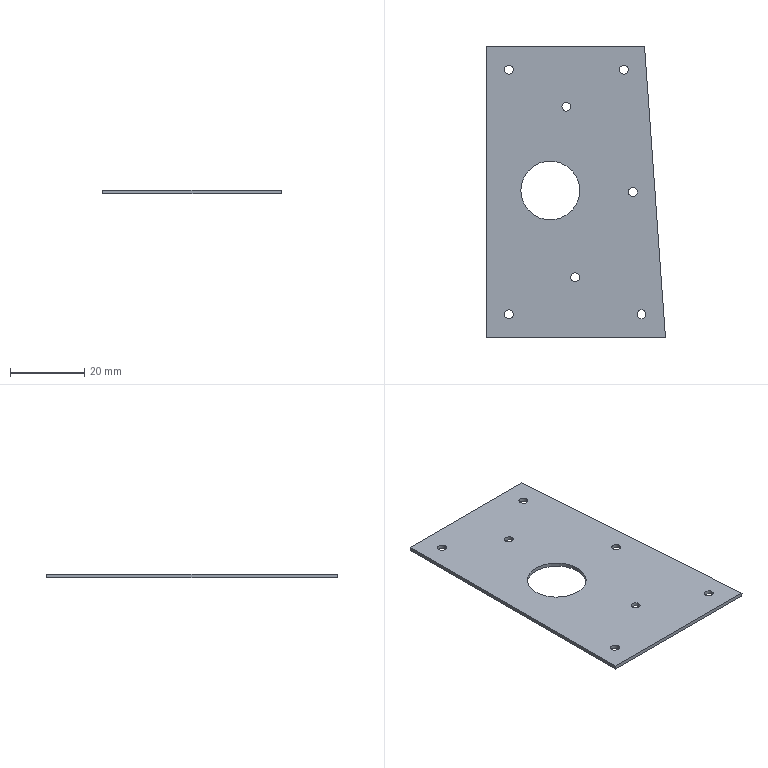Part | SolidWorks | features BaseBody 1 | 1 solid | 22 faces | box 48.271 x 78.4 x 1 mm | volume 3333 mm3 | cylinder 16 | plane 6 | commonest cylinder face diameters 2.4 x14 15.9 x2
STEP:
#1=CARTESIAN_POINT('',(25.15,40.,0.));
#2=VERTEX_POINT('',#1);
#3=CARTESIAN_POINT('',(9.25,40.,0.));
#4=VERTEX_POINT('',#3);
#5=CARTESIAN_POINT('',(17.2,40.,0.));
#6=DIRECTION('',(0.,0.,-1.));
#7=DIRECTION('',(1.,0.,0.));
#8=AXIS2_PLACEMENT_3D('',#5,#6,#7);
#9=CIRCLE('',#8,7.95);
#10=EDGE_CURVE('',#2,#4,#9,.T.);
#11=ORIENTED_EDGE('',*,*,#10,.T.);
#12=CARTESIAN_POINT('',(9.25,40.,1.));
#13=VERTEX_POINT('',#12);
#14=CARTESIAN_POINT('',(9.25,40.,0.));
#15=DIRECTION('',(0.,0.,1.));
#16=VECTOR('',#15,1000.);
#17=LINE('',#14,#16);
#18=EDGE_CURVE('',#4,#13,#17,.T.);
#19=ORIENTED_EDGE('',*,*,#18,.T.);
#20=CARTESIAN_POINT('',(25.15,40.,1.));
#21=VERTEX_POINT('',#20);
#22=CARTESIAN_POINT('',(17.2,40.,1.));
#23=DIRECTION('',(0.,0.,1.));
#24=DIRECTION('',(1.,0.,0.));
#25=AXIS2_PLACEMENT_3D('',#22,#23,#24);
#26=CIRCLE('',#25,7.95);
#27=EDGE_CURVE('',#13,#21,#26,.T.);
#28=ORIENTED_EDGE('',*,*,#27,.T.);
#29=CARTESIAN_POINT('',(25.15,40.,0.));
#30=DIRECTION('',(0.,0.,1.));
#31=VECTOR('',#30,1000.);
#32=LINE('',#29,#31);
#33=EDGE_CURVE('',#2,#21,#32,.T.);
#34=ORIENTED_EDGE('',*,*,#33,.F.);
#35=EDGE_LOOP('',(#11,#19,#28,#34));
#36=FACE_OUTER_BOUND('',#35,.T.);
#37=CARTESIAN_POINT('',(17.2,40.,0.));
#38=DIRECTION('',(0.,0.,1.));
#39=DIRECTION('',(1.,0.,0.));
#40=AXIS2_PLACEMENT_3D('',#37,#38,#39);
#41=CYLINDRICAL_SURFACE('',#40,7.95);
#42=ADVANCED_FACE('',(#36),#41,.F.);
#43=CARTESIAN_POINT('',(4.8,72.6,0.));
#44=VERTEX_POINT('',#43);
#45=CARTESIAN_POINT('',(7.2,72.6,0.));
#46=VERTEX_POINT('',#45);
#47=CARTESIAN_POINT('',(6.,72.6,0.));
#48=DIRECTION('',(0.,0.,1.));
#49=DIRECTION('',(1.,0.,0.));
#50=AXIS2_PLACEMENT_3D('',#47,#48,#49);
#51=CIRCLE('',#50,1.2);
#52=EDGE_CURVE('',#44,#46,#51,.T.);
#53=ORIENTED_EDGE('',*,*,#52,.F.);
#54=CARTESIAN_POINT('',(4.8,72.6,1.));
#55=VERTEX_POINT('',#54);
#56=CARTESIAN_POINT('',(4.8,72.6,0.));
#57=DIRECTION('',(0.,0.,1.));
#58=VECTOR('',#57,1000.);
#59=LINE('',#56,#58);
#60=EDGE_CURVE('',#44,#55,#59,.T.);
#61=ORIENTED_EDGE('',*,*,#60,.T.);
#62=CARTESIAN_POINT('',(7.2,72.6,1.));
#63=VERTEX_POINT('',#62);
#64=CARTESIAN_POINT('',(6.,72.6,1.));
#65=DIRECTION('',(0.,0.,1.));
#66=DIRECTION('',(1.,0.,0.));
#67=AXIS2_PLACEMENT_3D('',#64,#65,#66);
#68=CIRCLE('',#67,1.2);
#69=EDGE_CURVE('',#55,#63,#68,.T.);
#70=ORIENTED_EDGE('',*,*,#69,.T.);
#71=CARTESIAN_POINT('',(7.2,72.6,0.));
#72=DIRECTION('',(0.,0.,1.));
#73=VECTOR('',#72,1000.);
#74=LINE('',#71,#73);
#75=EDGE_CURVE('',#46,#63,#74,.T.);
#76=ORIENTED_EDGE('',*,*,#75,.F.);
#77=EDGE_LOOP('',(#53,#61,#70,#76));
#78=FACE_OUTER_BOUND('',#77,.T.);
#79=CARTESIAN_POINT('',(6.,72.6,0.));
#80=DIRECTION('',(0.,0.,1.));
#81=DIRECTION('',(1.,0.,0.));
#82=AXIS2_PLACEMENT_3D('',#79,#80,#81);
#83=CYLINDRICAL_SURFACE('',#82,1.2);
#84=ADVANCED_FACE('',(#78),#83,.F.);
#85=CARTESIAN_POINT('',(35.859,72.6,0.));
#86=VERTEX_POINT('',#85);
#87=CARTESIAN_POINT('',(38.259,72.6,0.));
#88=VERTEX_POINT('',#87);
#89=CARTESIAN_POINT('',(37.059,72.6,0.));
#90=DIRECTION('',(0.,0.,1.));
#91=DIRECTION('',(1.,0.,0.));
#92=AXIS2_PLACEMENT_3D('',#89,#90,#91);
#93=CIRCLE('',#92,1.2);
#94=EDGE_CURVE('',#86,#88,#93,.T.);
#95=ORIENTED_EDGE('',*,*,#94,.F.);
#96=CARTESIAN_POINT('',(35.859,72.6,1.));
#97=VERTEX_POINT('',#96);
#98=CARTESIAN_POINT('',(35.859,72.6,0.));
#99=DIRECTION('',(0.,0.,1.));
#100=VECTOR('',#99,1000.);
#101=LINE('',#98,#100);
#102=EDGE_CURVE('',#86,#97,#101,.T.);
#103=ORIENTED_EDGE('',*,*,#102,.T.);
#104=CARTESIAN_POINT('',(38.259,72.6,1.));
#105=VERTEX_POINT('',#104);
#106=CARTESIAN_POINT('',(37.059,72.6,1.));
#107=DIRECTION('',(0.,0.,1.));
#108=DIRECTION('',(1.,0.,0.));
#109=AXIS2_PLACEMENT_3D('',#106,#107,#108);
#110=CIRCLE('',#109,1.2);
#111=EDGE_CURVE('',#97,#105,#110,.T.);
#112=ORIENTED_EDGE('',*,*,#111,.T.);
#113=CARTESIAN_POINT('',(38.259,72.6,0.));
#114=DIRECTION('',(0.,0.,1.));
#115=VECTOR('',#114,1000.);
#116=LINE('',#113,#115);
#117=EDGE_CURVE('',#88,#105,#116,.T.);
#118=ORIENTED_EDGE('',*,*,#117,.F.);
#119=EDGE_LOOP('',(#95,#103,#112,#118));
#120=FACE_OUTER_BOUND('',#119,.T.);
#121=CARTESIAN_POINT('',(37.059,72.6,0.));
#122=DIRECTION('',(0.,0.,1.));
#123=DIRECTION('',(1.,0.,0.));
#124=AXIS2_PLACEMENT_3D('',#121,#122,#123);
#125=CYLINDRICAL_SURFACE('',#124,1.2);
#126=ADVANCED_FACE('',(#120),#125,.F.);
#127=CARTESIAN_POINT('',(4.8,6.6,0.));
#128=VERTEX_POINT('',#127);
#129=CARTESIAN_POINT('',(7.2,6.6,0.));
#130=VERTEX_POINT('',#129);
#131=CARTESIAN_POINT('',(6.,6.6,0.));
#132=DIRECTION('',(0.,0.,1.));
#133=DIRECTION('',(1.,0.,0.));
#134=AXIS2_PLACEMENT_3D('',#131,#132,#133);
#135=CIRCLE('',#134,1.2);
#136=EDGE_CURVE('',#128,#130,#135,.T.);
#137=ORIENTED_EDGE('',*,*,#136,.F.);
#138=CARTESIAN_POINT('',(4.8,6.6,1.));
#139=VERTEX_POINT('',#138);
#140=CARTESIAN_POINT('',(4.8,6.6,0.));
#141=DIRECTION('',(0.,0.,1.));
#142=VECTOR('',#141,1000.);
#143=LINE('',#140,#142);
#144=EDGE_CURVE('',#128,#139,#143,.T.);
#145=ORIENTED_EDGE('',*,*,#144,.T.);
#146=CARTESIAN_POINT('',(7.2,6.6,1.));
#147=VERTEX_POINT('',#146);
#148=CARTESIAN_POINT('',(6.,6.6,1.));
#149=DIRECTION('',(0.,0.,1.));
#150=DIRECTION('',(1.,0.,0.));
#151=AXIS2_PLACEMENT_3D('',#148,#149,#150);
#152=CIRCLE('',#151,1.2);
#153=EDGE_CURVE('',#139,#147,#152,.T.);
#154=ORIENTED_EDGE('',*,*,#153,.T.);
#155=CARTESIAN_POINT('',(7.2,6.6,0.));
#156=DIRECTION('',(0.,0.,1.));
#157=VECTOR('',#156,1000.);
#158=LINE('',#155,#157);
#159=EDGE_CURVE('',#130,#147,#158,.T.);
#160=ORIENTED_EDGE('',*,*,#159,.F.);
#161=EDGE_LOOP('',(#137,#145,#154,#160));
#162=FACE_OUTER_BOUND('',#161,.T.);
#163=CARTESIAN_POINT('',(6.,6.6,0.));
#164=DIRECTION('',(0.,0.,1.));
#165=DIRECTION('',(1.,0.,0.));
#166=AXIS2_PLACEMENT_3D('',#163,#164,#165);
#167=CYLINDRICAL_SURFACE('',#166,1.2);
#168=ADVANCED_FACE('',(#162),#167,.F.);
#169=CARTESIAN_POINT('',(40.609,6.6,0.));
#170=VERTEX_POINT('',#169);
#171=CARTESIAN_POINT('',(43.009,6.6,0.));
#172=VERTEX_POINT('',#171);
#173=CARTESIAN_POINT('',(41.809,6.6,0.));
#174=DIRECTION('',(0.,0.,1.));
#175=DIRECTION('',(1.,0.,0.));
#176=AXIS2_PLACEMENT_3D('',#173,#174,#175);
#177=CIRCLE('',#176,1.2);
#178=EDGE_CURVE('',#170,#172,#177,.T.);
#179=ORIENTED_EDGE('',*,*,#178,.F.);
#180=CARTESIAN_POINT('',(40.609,6.6,1.));
#181=VERTEX_POINT('',#180);
#182=CARTESIAN_POINT('',(40.609,6.6,0.));
#183=DIRECTION('',(0.,0.,1.));
#184=VECTOR('',#183,1000.);
#185=LINE('',#182,#184);
#186=EDGE_CURVE('',#170,#181,#185,.T.);
#187=ORIENTED_EDGE('',*,*,#186,.T.);
#188=CARTESIAN_POINT('',(43.009,6.6,1.));
#189=VERTEX_POINT('',#188);
#190=CARTESIAN_POINT('',(41.809,6.6,1.));
#191=DIRECTION('',(0.,0.,1.));
#192=DIRECTION('',(1.,0.,0.));
#193=AXIS2_PLACEMENT_3D('',#190,#191,#192);
#194=CIRCLE('',#193,1.2);
#195=EDGE_CURVE('',#181,#189,#194,.T.);
#196=ORIENTED_EDGE('',*,*,#195,.T.);
#197=CARTESIAN_POINT('',(43.009,6.6,0.));
#198=DIRECTION('',(0.,0.,1.));
#199=VECTOR('',#198,1000.);
#200=LINE('',#197,#199);
#201=EDGE_CURVE('',#172,#189,#200,.T.);
#202=ORIENTED_EDGE('',*,*,#201,.F.);
#203=EDGE_LOOP('',(#179,#187,#196,#202));
#204=FACE_OUTER_BOUND('',#203,.T.);
#205=CARTESIAN_POINT('',(41.809,6.6,0.));
#206=DIRECTION('',(0.,0.,1.));
#207=DIRECTION('',(1.,0.,0.));
#208=AXIS2_PLACEMENT_3D('',#205,#206,#207);
#209=CYLINDRICAL_SURFACE('',#208,1.2);
#210=ADVANCED_FACE('',(#204),#209,.F.);
#211=CARTESIAN_POINT('',(38.234,39.6,0.));
#212=VERTEX_POINT('',#211);
#213=CARTESIAN_POINT('',(40.634,39.6,0.));
#214=VERTEX_POINT('',#213);
#215=CARTESIAN_POINT('',(39.434,39.6,0.));
#216=DIRECTION('',(0.,0.,1.));
#217=DIRECTION('',(1.,0.,0.));
#218=AXIS2_PLACEMENT_3D('',#215,#216,#217);
#219=CIRCLE('',#218,1.2);
#220=EDGE_CURVE('',#212,#214,#219,.T.);
#221=ORIENTED_EDGE('',*,*,#220,.F.);
#222=CARTESIAN_POINT('',(38.234,39.6,1.));
#223=VERTEX_POINT('',#222);
#224=CARTESIAN_POINT('',(38.234,39.6,0.));
#225=DIRECTION('',(0.,0.,1.));
#226=VECTOR('',#225,1000.);
#227=LINE('',#224,#226);
#228=EDGE_CURVE('',#212,#223,#227,.T.);
#229=ORIENTED_EDGE('',*,*,#228,.T.);
#230=CARTESIAN_POINT('',(40.634,39.6,1.));
#231=VERTEX_POINT('',#230);
#232=CARTESIAN_POINT('',(39.434,39.6,1.));
#233=DIRECTION('',(0.,0.,1.));
#234=DIRECTION('',(1.,0.,0.));
#235=AXIS2_PLACEMENT_3D('',#232,#233,#234);
#236=CIRCLE('',#235,1.2);
#237=EDGE_CURVE('',#223,#231,#236,.T.);
#238=ORIENTED_EDGE('',*,*,#237,.T.);
#239=CARTESIAN_POINT('',(40.634,39.6,0.));
#240=DIRECTION('',(0.,0.,1.));
#241=VECTOR('',#240,1000.);
#242=LINE('',#239,#241);
#243=EDGE_CURVE('',#214,#231,#242,.T.);
#244=ORIENTED_EDGE('',*,*,#243,.F.);
#245=EDGE_LOOP('',(#221,#229,#238,#244));
#246=FACE_OUTER_BOUND('',#245,.T.);
#247=CARTESIAN_POINT('',(39.434,39.6,0.));
#248=DIRECTION('',(0.,0.,1.));
#249=DIRECTION('',(1.,0.,0.));
#250=AXIS2_PLACEMENT_3D('',#247,#248,#249);
#251=CYLINDRICAL_SURFACE('',#250,1.2);
#252=ADVANCED_FACE('',(#246),#251,.F.);
#253=CARTESIAN_POINT('',(22.705,16.6,0.));
#254=VERTEX_POINT('',#253);
#255=CARTESIAN_POINT('',(25.105,16.6,0.));
#256=VERTEX_POINT('',#255);
#257=CARTESIAN_POINT('',(23.905,16.6,0.));
#258=DIRECTION('',(0.,0.,1.));
#259=DIRECTION('',(1.,0.,0.));
#260=AXIS2_PLACEMENT_3D('',#257,#258,#259);
#261=CIRCLE('',#260,1.2);
#262=EDGE_CURVE('',#254,#256,#261,.T.);
#263=ORIENTED_EDGE('',*,*,#262,.F.);
#264=CARTESIAN_POINT('',(22.705,16.6,1.));
#265=VERTEX_POINT('',#264);
#266=CARTESIAN_POINT('',(22.705,16.6,0.));
#267=DIRECTION('',(0.,0.,1.));
#268=VECTOR('',#267,1000.);
#269=LINE('',#266,#268);
#270=EDGE_CURVE('',#254,#265,#269,.T.);
#271=ORIENTED_EDGE('',*,*,#270,.T.);
#272=CARTESIAN_POINT('',(25.105,16.6,1.));
#273=VERTEX_POINT('',#272);
#274=CARTESIAN_POINT('',(23.905,16.6,1.));
#275=DIRECTION('',(0.,0.,1.));
#276=DIRECTION('',(1.,0.,0.));
#277=AXIS2_PLACEMENT_3D('',#274,#275,#276);
#278=CIRCLE('',#277,1.2);
#279=EDGE_CURVE('',#265,#273,#278,.T.);
#280=ORIENTED_EDGE('',*,*,#279,.T.);
#281=CARTESIAN_POINT('',(25.105,16.6,0.));
#282=DIRECTION('',(0.,0.,1.));
#283=VECTOR('',#282,1000.);
#284=LINE('',#281,#283);
#285=EDGE_CURVE('',#256,#273,#284,.T.);
#286=ORIENTED_EDGE('',*,*,#285,.F.);
#287=EDGE_LOOP('',(#263,#271,#280,#286));
#288=FACE_OUTER_BOUND('',#287,.T.);
#289=CARTESIAN_POINT('',(23.905,16.6,0.));
#290=DIRECTION('',(0.,0.,1.));
#291=DIRECTION('',(1.,0.,0.));
#292=AXIS2_PLACEMENT_3D('',#289,#290,#291);
#293=CYLINDRICAL_SURFACE('',#292,1.2);
#294=ADVANCED_FACE('',(#288),#293,.F.);
#295=CARTESIAN_POINT('',(20.33,62.6,0.));
#296=VERTEX_POINT('',#295);
#297=CARTESIAN_POINT('',(22.73,62.6,0.));
#298=VERTEX_POINT('',#297);
#299=CARTESIAN_POINT('',(21.53,62.6,0.));
#300=DIRECTION('',(0.,0.,1.));
#301=DIRECTION('',(1.,0.,0.));
#302=AXIS2_PLACEMENT_3D('',#299,#300,#301);
#303=CIRCLE('',#302,1.2);
#304=EDGE_CURVE('',#296,#298,#303,.T.);
#305=ORIENTED_EDGE('',*,*,#304,.F.);
#306=CARTESIAN_POINT('',(20.33,62.6,1.));
#307=VERTEX_POINT('',#306);
#308=CARTESIAN_POINT('',(20.33,62.6,0.));
#309=DIRECTION('',(0.,0.,1.));
#310=VECTOR('',#309,1000.);
#311=LINE('',#308,#310);
#312=EDGE_CURVE('',#296,#307,#311,.T.);
#313=ORIENTED_EDGE('',*,*,#312,.T.);
#314=CARTESIAN_POINT('',(22.73,62.6,1.));
#315=VERTEX_POINT('',#314);
#316=CARTESIAN_POINT('',(21.53,62.6,1.));
#317=DIRECTION('',(0.,0.,1.));
#318=DIRECTION('',(1.,0.,0.));
#319=AXIS2_PLACEMENT_3D('',#316,#317,#318);
#320=CIRCLE('',#319,1.2);
#321=EDGE_CURVE('',#307,#315,#320,.T.);
#322=ORIENTED_EDGE('',*,*,#321,.T.);
#323=CARTESIAN_POINT('',(22.73,62.6,0.));
#324=DIRECTION('',(0.,0.,1.));
#325=VECTOR('',#324,1000.);
#326=LINE('',#323,#325);
#327=EDGE_CURVE('',#298,#315,#326,.T.);
#328=ORIENTED_EDGE('',*,*,#327,.F.);
#329=EDGE_LOOP('',(#305,#313,#322,#328));
#330=FACE_OUTER_BOUND('',#329,.T.);
#331=CARTESIAN_POINT('',(21.53,62.6,0.));
#332=DIRECTION('',(0.,0.,1.));
#333=DIRECTION('',(1.,0.,0.));
#334=AXIS2_PLACEMENT_3D('',#331,#332,#333);
#335=CYLINDRICAL_SURFACE('',#334,1.2);
#336=ADVANCED_FACE('',(#330),#335,.F.);
#337=ORIENTED_EDGE('',*,*,#18,.F.);
#338=CARTESIAN_POINT('',(17.2,40.,0.));
#339=DIRECTION('',(0.,0.,-1.));
#340=DIRECTION('',(1.,0.,0.));
#341=AXIS2_PLACEMENT_3D('',#338,#339,#340);
#342=CIRCLE('',#341,7.95);
#343=EDGE_CURVE('',#4,#2,#342,.T.);
#344=ORIENTED_EDGE('',*,*,#343,.T.);
#345=ORIENTED_EDGE('',*,*,#33,.T.);
#346=CARTESIAN_POINT('',(17.2,40.,1.));
#347=DIRECTION('',(0.,0.,1.));
#348=DIRECTION('',(1.,0.,0.));
#349=AXIS2_PLACEMENT_3D('',#346,#347,#348);
#350=CIRCLE('',#349,7.95);
#351=EDGE_CURVE('',#21,#13,#350,.T.);
#352=ORIENTED_EDGE('',*,*,#351,.T.);
#353=EDGE_LOOP('',(#337,#344,#345,#352));
#354=FACE_OUTER_BOUND('',#353,.T.);
#355=CARTESIAN_POINT('',(17.2,40.,0.));
#356=DIRECTION('',(0.,0.,1.));
#357=DIRECTION('',(1.,0.,0.));
#358=AXIS2_PLACEMENT_3D('',#355,#356,#357);
#359=CYLINDRICAL_SURFACE('',#358,7.95);
#360=ADVANCED_FACE('',(#354),#359,.F.);
#361=CARTESIAN_POINT('',(6.,72.6,1.));
#362=DIRECTION('',(0.,0.,1.));
#363=DIRECTION('',(1.,0.,0.));
#364=AXIS2_PLACEMENT_3D('',#361,#362,#363);
#365=CIRCLE('',#364,1.2);
#366=EDGE_CURVE('',#63,#55,#365,.T.);
#367=ORIENTED_EDGE('',*,*,#366,.F.);
#368=ORIENTED_EDGE('',*,*,#69,.F.);
#369=EDGE_LOOP('',(#367,#368));
#370=FACE_BOUND('',#369,.T.);
#371=CARTESIAN_POINT('',(37.059,72.6,1.));
#372=DIRECTION('',(0.,0.,1.));
#373=DIRECTION('',(1.,0.,0.));
#374=AXIS2_PLACEMENT_3D('',#371,#372,#373);
#375=CIRCLE('',#374,1.2);
#376=EDGE_CURVE('',#105,#97,#375,.T.);
#377=ORIENTED_EDGE('',*,*,#376,.F.);
#378=ORIENTED_EDGE('',*,*,#111,.F.);
#379=EDGE_LOOP('',(#377,#378));
#380=FACE_BOUND('',#379,.T.);
#381=CARTESIAN_POINT('',(6.,6.6,1.));
#382=DIRECTION('',(0.,0.,1.));
#383=DIRECTION('',(1.,0.,0.));
#384=AXIS2_PLACEMENT_3D('',#381,#382,#383);
#385=CIRCLE('',#384,1.2);
#386=EDGE_CURVE('',#147,#139,#385,.T.);
#387=ORIENTED_EDGE('',*,*,#386,.F.);
#388=ORIENTED_EDGE('',*,*,#153,.F.);
#389=EDGE_LOOP('',(#387,#388));
#390=FACE_BOUND('',#389,.T.);
#391=CARTESIAN_POINT('',(41.809,6.6,1.));
#392=DIRECTION('',(0.,0.,1.));
#393=DIRECTION('',(1.,0.,0.));
#394=AXIS2_PLACEMENT_3D('',#391,#392,#393);
#395=CIRCLE('',#394,1.2);
#396=EDGE_CURVE('',#189,#181,#395,.T.);
#397=ORIENTED_EDGE('',*,*,#396,.F.);
#398=ORIENTED_EDGE('',*,*,#195,.F.);
#399=EDGE_LOOP('',(#397,#398));
#400=FACE_BOUND('',#399,.T.);
#401=CARTESIAN_POINT('',(39.434,39.6,1.));
#402=DIRECTION('',(0.,0.,1.));
#403=DIRECTION('',(1.,0.,0.));
#404=AXIS2_PLACEMENT_3D('',#401,#402,#403);
#405=CIRCLE('',#404,1.2);
#406=EDGE_CURVE('',#231,#223,#405,.T.);
#407=ORIENTED_EDGE('',*,*,#406,.F.);
#408=ORIENTED_EDGE('',*,*,#237,.F.);
#409=EDGE_LOOP('',(#407,#408));
#410=FACE_BOUND('',#409,.T.);
#411=CARTESIAN_POINT('',(23.905,16.6,1.));
#412=DIRECTION('',(0.,0.,1.));
#413=DIRECTION('',(1.,0.,0.));
#414=AXIS2_PLACEMENT_3D('',#411,#412,#413);
#415=CIRCLE('',#414,1.2);
#416=EDGE_CURVE('',#273,#265,#415,.T.);
#417=ORIENTED_EDGE('',*,*,#416,.F.);
#418=ORIENTED_EDGE('',*,*,#279,.F.);
#419=EDGE_LOOP('',(#417,#418));
#420=FACE_BOUND('',#419,.T.);
#421=CARTESIAN_POINT('',(21.53,62.6,1.));
#422=DIRECTION('',(0.,0.,1.));
#423=DIRECTION('',(1.,0.,0.));
#424=AXIS2_PLACEMENT_3D('',#421,#422,#423);
#425=CIRCLE('',#424,1.2);
#426=EDGE_CURVE('',#315,#307,#425,.T.);
#427=ORIENTED_EDGE('',*,*,#426,.F.);
#428=ORIENTED_EDGE('',*,*,#321,.F.);
#429=EDGE_LOOP('',(#427,#428));
#430=FACE_BOUND('',#429,.T.);
#431=ORIENTED_EDGE('',*,*,#351,.F.);
#432=ORIENTED_EDGE('',*,*,#27,.F.);
#433=EDGE_LOOP('',(#431,#432));
#434=FACE_BOUND('',#433,.T.);
#435=CARTESIAN_POINT('',(48.271,0.4,1.));
#436=VERTEX_POINT('',#435);
#437=CARTESIAN_POINT('',(0.,0.4,1.));
#438=VERTEX_POINT('',#437);
#439=CARTESIAN_POINT('',(24.28,0.4,1.));
#440=DIRECTION('',(-1.,0.,0.));
#441=VECTOR('',#440,1000.);
#442=LINE('',#439,#441);
#443=EDGE_CURVE('',#436,#438,#442,.T.);
#444=ORIENTED_EDGE('',*,*,#443,.F.);
#445=CARTESIAN_POINT('',(42.629,78.8,1.));
#446=VERTEX_POINT('',#445);
#447=CARTESIAN_POINT('',(42.629,78.8,1.));
#448=DIRECTION('',(0.07178,-0.9974,0.));
#449=VECTOR('',#448,1000.);
#450=LINE('',#447,#449);
#451=EDGE_CURVE('',#446,#436,#450,.T.);
#452=ORIENTED_EDGE('',*,*,#451,.F.);
#453=CARTESIAN_POINT('',(0.,78.8,1.));
#454=VERTEX_POINT('',#453);
#455=CARTESIAN_POINT('',(24.28,78.8,1.));
#456=DIRECTION('',(1.,0.,0.));
#457=VECTOR('',#456,1000.);
#458=LINE('',#455,#457);
#459=EDGE_CURVE('',#454,#446,#458,.T.);
#460=ORIENTED_EDGE('',*,*,#459,.F.);
#461=CARTESIAN_POINT('',(0.,39.6,1.));
#462=DIRECTION('',(0.,1.,0.));
#463=VECTOR('',#462,1000.);
#464=LINE('',#461,#463);
#465=EDGE_CURVE('',#438,#454,#464,.T.);
#466=ORIENTED_EDGE('',*,*,#465,.F.);
#467=EDGE_LOOP('',(#444,#452,#460,#466));
#468=FACE_OUTER_BOUND('',#467,.T.);
#469=CARTESIAN_POINT('',(48.561,0.4,1.));
#470=DIRECTION('',(0.,0.,-1.));
#471=DIRECTION('',(-1.,0.,0.));
#472=AXIS2_PLACEMENT_3D('',#469,#470,#471);
#473=PLANE('',#472);
#474=ADVANCED_FACE('',(#370,#380,#390,#400,#410,#420,#430,#434,#468),#473,.F.);
#475=CARTESIAN_POINT('',(6.,72.6,0.));
#476=DIRECTION('',(0.,0.,1.));
#477=DIRECTION('',(1.,0.,0.));
#478=AXIS2_PLACEMENT_3D('',#475,#476,#477);
#479=CIRCLE('',#478,1.2);
#480=EDGE_CURVE('',#46,#44,#479,.T.);
#481=ORIENTED_EDGE('',*,*,#480,.T.);
#482=ORIENTED_EDGE('',*,*,#52,.T.);
#483=EDGE_LOOP('',(#481,#482));
#484=FACE_BOUND('',#483,.T.);
#485=CARTESIAN_POINT('',(37.059,72.6,0.));
#486=DIRECTION('',(0.,0.,1.));
#487=DIRECTION('',(1.,0.,0.));
#488=AXIS2_PLACEMENT_3D('',#485,#486,#487);
#489=CIRCLE('',#488,1.2);
#490=EDGE_CURVE('',#88,#86,#489,.T.);
#491=ORIENTED_EDGE('',*,*,#490,.T.);
#492=ORIENTED_EDGE('',*,*,#94,.T.);
#493=EDGE_LOOP('',(#491,#492));
#494=FACE_BOUND('',#493,.T.);
#495=CARTESIAN_POINT('',(6.,6.6,0.));
#496=DIRECTION('',(0.,0.,1.));
#497=DIRECTION('',(1.,0.,0.));
#498=AXIS2_PLACEMENT_3D('',#495,#496,#497);
#499=CIRCLE('',#498,1.2);
#500=EDGE_CURVE('',#130,#128,#499,.T.);
#501=ORIENTED_EDGE('',*,*,#500,.T.);
#502=ORIENTED_EDGE('',*,*,#136,.T.);
#503=EDGE_LOOP('',(#501,#502));
#504=FACE_BOUND('',#503,.T.);
#505=CARTESIAN_POINT('',(41.809,6.6,0.));
#506=DIRECTION('',(0.,0.,1.));
#507=DIRECTION('',(1.,0.,0.));
#508=AXIS2_PLACEMENT_3D('',#505,#506,#507);
#509=CIRCLE('',#508,1.2);
#510=EDGE_CURVE('',#172,#170,#509,.T.);
#511=ORIENTED_EDGE('',*,*,#510,.T.);
#512=ORIENTED_EDGE('',*,*,#178,.T.);
#513=EDGE_LOOP('',(#511,#512));
#514=FACE_BOUND('',#513,.T.);
#515=CARTESIAN_POINT('',(39.434,39.6,0.));
#516=DIRECTION('',(0.,0.,1.));
#517=DIRECTION('',(1.,0.,0.));
#518=AXIS2_PLACEMENT_3D('',#515,#516,#517);
#519=CIRCLE('',#518,1.2);
#520=EDGE_CURVE('',#214,#212,#519,.T.);
#521=ORIENTED_EDGE('',*,*,#520,.T.);
#522=ORIENTED_EDGE('',*,*,#220,.T.);
#523=EDGE_LOOP('',(#521,#522));
#524=FACE_BOUND('',#523,.T.);
#525=CARTESIAN_POINT('',(23.905,16.6,0.));
#526=DIRECTION('',(0.,0.,1.));
#527=DIRECTION('',(1.,0.,0.));
#528=AXIS2_PLACEMENT_3D('',#525,#526,#527);
#529=CIRCLE('',#528,1.2);
#530=EDGE_CURVE('',#256,#254,#529,.T.);
#531=ORIENTED_EDGE('',*,*,#530,.T.);
#532=ORIENTED_EDGE('',*,*,#262,.T.);
#533=EDGE_LOOP('',(#531,#532));
#534=FACE_BOUND('',#533,.T.);
#535=CARTESIAN_POINT('',(21.53,62.6,0.));
#536=DIRECTION('',(0.,0.,1.));
#537=DIRECTION('',(1.,0.,0.));
#538=AXIS2_PLACEMENT_3D('',#535,#536,#537);
#539=CIRCLE('',#538,1.2);
#540=EDGE_CURVE('',#298,#296,#539,.T.);
#541=ORIENTED_EDGE('',*,*,#540,.T.);
#542=ORIENTED_EDGE('',*,*,#304,.T.);
#543=EDGE_LOOP('',(#541,#542));
#544=FACE_BOUND('',#543,.T.);
#545=ORIENTED_EDGE('',*,*,#10,.F.);
#546=ORIENTED_EDGE('',*,*,#343,.F.);
#547=EDGE_LOOP('',(#545,#546));
#548=FACE_BOUND('',#547,.T.);
#549=CARTESIAN_POINT('',(0.,78.8,0.));
#550=VERTEX_POINT('',#549);
#551=CARTESIAN_POINT('',(42.629,78.8,0.));
#552=VERTEX_POINT('',#551);
#553=CARTESIAN_POINT('',(24.28,78.8,0.));
#554=DIRECTION('',(1.,0.,0.));
#555=VECTOR('',#554,1000.);
#556=LINE('',#553,#555);
#557=EDGE_CURVE('',#550,#552,#556,.T.);
#558=ORIENTED_EDGE('',*,*,#557,.T.);
#559=CARTESIAN_POINT('',(48.271,0.4,0.));
#560=VERTEX_POINT('',#559);
#561=CARTESIAN_POINT('',(42.629,78.8,0.));
#562=DIRECTION('',(0.07178,-0.9974,0.));
#563=VECTOR('',#562,1000.);
#564=LINE('',#561,#563);
#565=EDGE_CURVE('',#552,#560,#564,.T.);
#566=ORIENTED_EDGE('',*,*,#565,.T.);
#567=CARTESIAN_POINT('',(0.,0.4,0.));
#568=VERTEX_POINT('',#567);
#569=CARTESIAN_POINT('',(24.28,0.4,0.));
#570=DIRECTION('',(-1.,0.,0.));
#571=VECTOR('',#570,1000.);
#572=LINE('',#569,#571);
#573=EDGE_CURVE('',#560,#568,#572,.T.);
#574=ORIENTED_EDGE('',*,*,#573,.T.);
#575=CARTESIAN_POINT('',(0.,39.6,0.));
#576=DIRECTION('',(0.,1.,0.));
#577=VECTOR('',#576,1000.);
#578=LINE('',#575,#577);
#579=EDGE_CURVE('',#568,#550,#578,.T.);
#580=ORIENTED_EDGE('',*,*,#579,.T.);
#581=EDGE_LOOP('',(#558,#566,#574,#580));
#582=FACE_OUTER_BOUND('',#581,.T.);
#583=CARTESIAN_POINT('',(48.561,0.4,0.));
#584=DIRECTION('',(0.,0.,-1.));
#585=DIRECTION('',(-1.,0.,0.));
#586=AXIS2_PLACEMENT_3D('',#583,#584,#585);
#587=PLANE('',#586);
#588=ADVANCED_FACE('',(#484,#494,#504,#514,#524,#534,#544,#548,#582),#587,.T.);
#589=ORIENTED_EDGE('',*,*,#60,.F.);
#590=ORIENTED_EDGE('',*,*,#480,.F.);
#591=ORIENTED_EDGE('',*,*,#75,.T.);
#592=ORIENTED_EDGE('',*,*,#366,.T.);
#593=EDGE_LOOP('',(#589,#590,#591,#592));
#594=FACE_OUTER_BOUND('',#593,.T.);
#595=CARTESIAN_POINT('',(6.,72.6,0.));
#596=DIRECTION('',(0.,0.,1.));
#597=DIRECTION('',(1.,0.,0.));
#598=AXIS2_PLACEMENT_3D('',#595,#596,#597);
#599=CYLINDRICAL_SURFACE('',#598,1.2);
#600=ADVANCED_FACE('',(#594),#599,.F.);
#601=ORIENTED_EDGE('',*,*,#102,.F.);
#602=ORIENTED_EDGE('',*,*,#490,.F.);
#603=ORIENTED_EDGE('',*,*,#117,.T.);
#604=ORIENTED_EDGE('',*,*,#376,.T.);
#605=EDGE_LOOP('',(#601,#602,#603,#604));
#606=FACE_OUTER_BOUND('',#605,.T.);
#607=CARTESIAN_POINT('',(37.059,72.6,0.));
#608=DIRECTION('',(0.,0.,1.));
#609=DIRECTION('',(1.,0.,0.));
#610=AXIS2_PLACEMENT_3D('',#607,#608,#609);
#611=CYLINDRICAL_SURFACE('',#610,1.2);
#612=ADVANCED_FACE('',(#606),#611,.F.);
#613=ORIENTED_EDGE('',*,*,#144,.F.);
#614=ORIENTED_EDGE('',*,*,#500,.F.);
#615=ORIENTED_EDGE('',*,*,#159,.T.);
#616=ORIENTED_EDGE('',*,*,#386,.T.);
#617=EDGE_LOOP('',(#613,#614,#615,#616));
#618=FACE_OUTER_BOUND('',#617,.T.);
#619=CARTESIAN_POINT('',(6.,6.6,0.));
#620=DIRECTION('',(0.,0.,1.));
#621=DIRECTION('',(1.,0.,0.));
#622=AXIS2_PLACEMENT_3D('',#619,#620,#621);
#623=CYLINDRICAL_SURFACE('',#622,1.2);
#624=ADVANCED_FACE('',(#618),#623,.F.);
#625=ORIENTED_EDGE('',*,*,#186,.F.);
#626=ORIENTED_EDGE('',*,*,#510,.F.);
#627=ORIENTED_EDGE('',*,*,#201,.T.);
#628=ORIENTED_EDGE('',*,*,#396,.T.);
#629=EDGE_LOOP('',(#625,#626,#627,#628));
#630=FACE_OUTER_BOUND('',#629,.T.);
#631=CARTESIAN_POINT('',(41.809,6.6,0.));
#632=DIRECTION('',(0.,0.,1.));
#633=DIRECTION('',(1.,0.,0.));
#634=AXIS2_PLACEMENT_3D('',#631,#632,#633);
#635=CYLINDRICAL_SURFACE('',#634,1.2);
#636=ADVANCED_FACE('',(#630),#635,.F.);
#637=ORIENTED_EDGE('',*,*,#228,.F.);
#638=ORIENTED_EDGE('',*,*,#520,.F.);
#639=ORIENTED_EDGE('',*,*,#243,.T.);
#640=ORIENTED_EDGE('',*,*,#406,.T.);
#641=EDGE_LOOP('',(#637,#638,#639,#640));
#642=FACE_OUTER_BOUND('',#641,.T.);
#643=CARTESIAN_POINT('',(39.434,39.6,0.));
#644=DIRECTION('',(0.,0.,1.));
#645=DIRECTION('',(1.,0.,0.));
#646=AXIS2_PLACEMENT_3D('',#643,#644,#645);
#647=CYLINDRICAL_SURFACE('',#646,1.2);
#648=ADVANCED_FACE('',(#642),#647,.F.);
#649=ORIENTED_EDGE('',*,*,#270,.F.);
#650=ORIENTED_EDGE('',*,*,#530,.F.);
#651=ORIENTED_EDGE('',*,*,#285,.T.);
#652=ORIENTED_EDGE('',*,*,#416,.T.);
#653=EDGE_LOOP('',(#649,#650,#651,#652));
#654=FACE_OUTER_BOUND('',#653,.T.);
#655=CARTESIAN_POINT('',(23.905,16.6,0.));
#656=DIRECTION('',(0.,0.,1.));
#657=DIRECTION('',(1.,0.,0.));
#658=AXIS2_PLACEMENT_3D('',#655,#656,#657);
#659=CYLINDRICAL_SURFACE('',#658,1.2);
#660=ADVANCED_FACE('',(#654),#659,.F.);
#661=ORIENTED_EDGE('',*,*,#312,.F.);
#662=ORIENTED_EDGE('',*,*,#540,.F.);
#663=ORIENTED_EDGE('',*,*,#327,.T.);
#664=ORIENTED_EDGE('',*,*,#426,.T.);
#665=EDGE_LOOP('',(#661,#662,#663,#664));
#666=FACE_OUTER_BOUND('',#665,.T.);
#667=CARTESIAN_POINT('',(21.53,62.6,0.));
#668=DIRECTION('',(0.,0.,1.));
#669=DIRECTION('',(1.,0.,0.));
#670=AXIS2_PLACEMENT_3D('',#667,#668,#669);
#671=CYLINDRICAL_SURFACE('',#670,1.2);
#672=ADVANCED_FACE('',(#666),#671,.F.);
#673=CARTESIAN_POINT('',(0.,0.4,0.5));
#674=DIRECTION('',(0.,0.,-1.));
#675=VECTOR('',#674,1000.);
#676=LINE('',#673,#675);
#677=EDGE_CURVE('',#438,#568,#676,.T.);
#678=ORIENTED_EDGE('',*,*,#677,.F.);
#679=ORIENTED_EDGE('',*,*,#465,.T.);
#680=CARTESIAN_POINT('',(0.,78.8,0.5));
#681=DIRECTION('',(0.,0.,1.));
#682=VECTOR('',#681,1000.);
#683=LINE('',#680,#682);
#684=EDGE_CURVE('',#550,#454,#683,.T.);
#685=ORIENTED_EDGE('',*,*,#684,.F.);
#686=ORIENTED_EDGE('',*,*,#579,.F.);
#687=EDGE_LOOP('',(#678,#679,#685,#686));
#688=FACE_OUTER_BOUND('',#687,.T.);
#689=CARTESIAN_POINT('',(0.,0.4,1.));
#690=DIRECTION('',(1.,0.,0.));
#691=DIRECTION('',(0.,0.,-1.));
#692=AXIS2_PLACEMENT_3D('',#689,#690,#691);
#693=PLANE('',#692);
#694=ADVANCED_FACE('',(#688),#693,.F.);
#695=CARTESIAN_POINT('',(48.271,0.4,0.5));
#696=DIRECTION('',(0.,0.,-1.));
#697=VECTOR('',#696,1000.);
#698=LINE('',#695,#697);
#699=EDGE_CURVE('',#436,#560,#698,.T.);
#700=ORIENTED_EDGE('',*,*,#699,.F.);
#701=ORIENTED_EDGE('',*,*,#443,.T.);
#702=ORIENTED_EDGE('',*,*,#677,.T.);
#703=ORIENTED_EDGE('',*,*,#573,.F.);
#704=EDGE_LOOP('',(#700,#701,#702,#703));
#705=FACE_OUTER_BOUND('',#704,.T.);
#706=CARTESIAN_POINT('',(0.,0.4,0.));
#707=DIRECTION('',(0.,1.,0.));
#708=DIRECTION('',(0.,0.,1.));
#709=AXIS2_PLACEMENT_3D('',#706,#707,#708);
#710=PLANE('',#709);
#711=ADVANCED_FACE('',(#705),#710,.F.);
#712=ORIENTED_EDGE('',*,*,#699,.T.);
#713=ORIENTED_EDGE('',*,*,#565,.F.);
#714=CARTESIAN_POINT('',(42.629,78.8,0.5));
#715=DIRECTION('',(0.,0.,-1.));
#716=VECTOR('',#715,1000.);
#717=LINE('',#714,#716);
#718=EDGE_CURVE('',#446,#552,#717,.T.);
#719=ORIENTED_EDGE('',*,*,#718,.F.);
#720=ORIENTED_EDGE('',*,*,#451,.T.);
#721=EDGE_LOOP('',(#712,#713,#719,#720));
#722=FACE_OUTER_BOUND('',#721,.T.);
#723=CARTESIAN_POINT('',(42.629,78.8,0.));
#724=DIRECTION('',(-0.9974,-0.07178,0.));
#725=DIRECTION('',(0.07178,-0.9974,0.));
#726=AXIS2_PLACEMENT_3D('',#723,#724,#725);
#727=PLANE('',#726);
#728=ADVANCED_FACE('',(#722),#727,.F.);
#729=ORIENTED_EDGE('',*,*,#718,.T.);
#730=ORIENTED_EDGE('',*,*,#557,.F.);
#731=ORIENTED_EDGE('',*,*,#684,.T.);
#732=ORIENTED_EDGE('',*,*,#459,.T.);
#733=EDGE_LOOP('',(#729,#730,#731,#732));
#734=FACE_OUTER_BOUND('',#733,.T.);
#735=CARTESIAN_POINT('',(0.,78.8,1.));
#736=DIRECTION('',(0.,-1.,0.));
#737=DIRECTION('',(0.,0.,-1.));
#738=AXIS2_PLACEMENT_3D('',#735,#736,#737);
#739=PLANE('',#738);
#740=ADVANCED_FACE('',(#734),#739,.F.);
#741=CLOSED_SHELL('',(#42,#84,#126,#168,#210,#252,#294,#336,#360,#474,#588,#600,#612,#624,#636,#648,#660,#672,#694,#711,#728,#740));
#742=MANIFOLD_SOLID_BREP('',#741);
#743=CARTESIAN_POINT('',(0.,0.,0.));
#744=DIRECTION('',(0.,0.,1.));
#745=DIRECTION('',(1.,0.,0.));
#746=AXIS2_PLACEMENT_3D('',#743,#744,#745);
#747=(LENGTH_UNIT()NAMED_UNIT(*)SI_UNIT(.MILLI.,.METRE.));
#748=UNCERTAINTY_MEASURE_WITH_UNIT(LENGTH_MEASURE(0.00001),#747,'','');
#749=(NAMED_UNIT(*)PLANE_ANGLE_UNIT()SI_UNIT($,.RADIAN.));
#750=(NAMED_UNIT(*)SI_UNIT($,.STERADIAN.)SOLID_ANGLE_UNIT());
#751=(GEOMETRIC_REPRESENTATION_CONTEXT(3)GLOBAL_UNCERTAINTY_ASSIGNED_CONTEXT((#748))GLOBAL_UNIT_ASSIGNED_CONTEXT((#747,#749,#750))REPRESENTATION_CONTEXT('',''));
#752=ADVANCED_BREP_SHAPE_REPRESENTATION('',(#742,#746),#751);